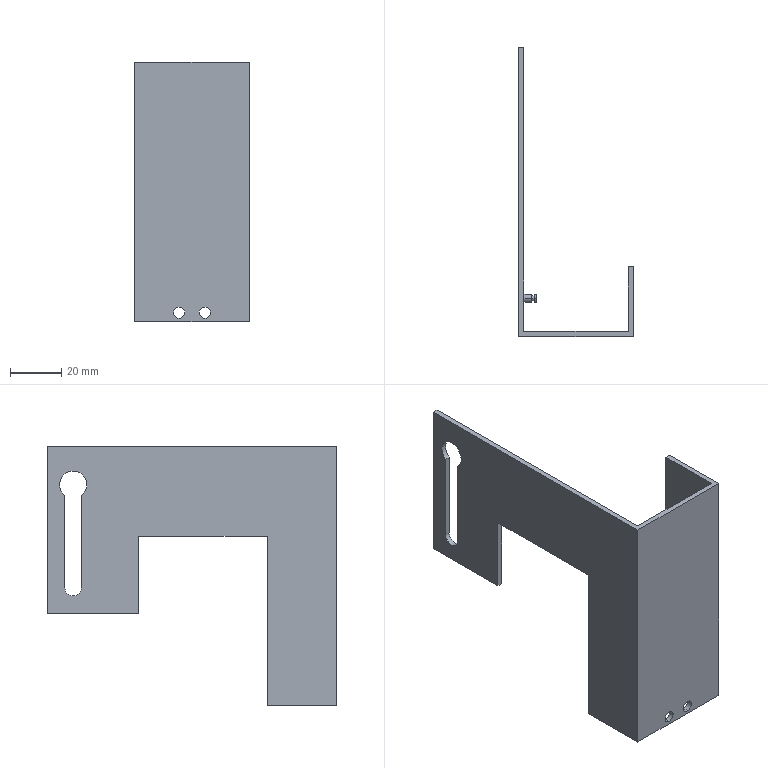Part | SolidWorks | features BaseBody 1 | 1 solid | 32 faces | box 44.5 x 112.5 x 101 mm | volume 26509 mm3 | plane 19 | cylinder 13 | commonest cylinder face diameters 3 x4 4.4 x4 2 x2 10.6 x2 6.5 x1
STEP:
#1=CARTESIAN_POINT('',(901.696,-4295.973,965.271));
#2=VERTEX_POINT('',#1);
#3=CARTESIAN_POINT('',(901.696,-4292.723,955.785));
#4=VERTEX_POINT('',#3);
#5=CARTESIAN_POINT('',(901.696,-4295.973,959.971));
#6=DIRECTION('',(-1.,0.,0.));
#7=DIRECTION('',(0.,0.,1.));
#8=AXIS2_PLACEMENT_3D('',#5,#6,#7);
#9=CIRCLE('',#8,5.3);
#10=EDGE_CURVE('',#2,#4,#9,.T.);
#11=ORIENTED_EDGE('',*,*,#10,.F.);
#12=CARTESIAN_POINT('',(899.696,-4295.973,965.271));
#13=VERTEX_POINT('',#12);
#14=CARTESIAN_POINT('',(922.28,-4295.973,965.271));
#15=DIRECTION('',(-1.,0.,0.));
#16=VECTOR('',#15,1000.);
#17=LINE('',#14,#16);
#18=EDGE_CURVE('',#2,#13,#17,.T.);
#19=ORIENTED_EDGE('',*,*,#18,.T.);
#20=CARTESIAN_POINT('',(899.696,-4292.723,955.785));
#21=VERTEX_POINT('',#20);
#22=CARTESIAN_POINT('',(899.696,-4295.973,959.971));
#23=DIRECTION('',(1.,0.,0.));
#24=DIRECTION('',(0.,0.,1.));
#25=AXIS2_PLACEMENT_3D('',#22,#23,#24);
#26=CIRCLE('',#25,5.3);
#27=EDGE_CURVE('',#21,#13,#26,.T.);
#28=ORIENTED_EDGE('',*,*,#27,.F.);
#29=CARTESIAN_POINT('',(973.716,-4292.723,955.785));
#30=DIRECTION('',(1.,0.,0.));
#31=VECTOR('',#30,1000.);
#32=LINE('',#29,#31);
#33=EDGE_CURVE('',#21,#4,#32,.T.);
#34=ORIENTED_EDGE('',*,*,#33,.T.);
#35=EDGE_LOOP('',(#11,#19,#28,#34));
#36=FACE_OUTER_BOUND('',#35,.T.);
#37=CARTESIAN_POINT('',(922.28,-4295.973,959.971));
#38=DIRECTION('',(-1.,0.,0.));
#39=DIRECTION('',(0.,0.,1.));
#40=AXIS2_PLACEMENT_3D('',#37,#38,#39);
#41=CYLINDRICAL_SURFACE('',#40,5.3);
#42=ADVANCED_FACE('',(#36),#41,.F.);
#43=CARTESIAN_POINT('',(916.941,-4396.473,879.671));
#44=VERTEX_POINT('',#43);
#45=CARTESIAN_POINT('',(916.941,-4396.473,875.271));
#46=VERTEX_POINT('',#45);
#47=CARTESIAN_POINT('',(916.941,-4396.473,877.471));
#48=DIRECTION('',(0.,-1.,0.));
#49=DIRECTION('',(0.,0.,-1.));
#50=AXIS2_PLACEMENT_3D('',#47,#48,#49);
#51=CIRCLE('',#50,2.2);
#52=EDGE_CURVE('',#44,#46,#51,.T.);
#53=ORIENTED_EDGE('',*,*,#52,.F.);
#54=CARTESIAN_POINT('',(916.941,-4398.473,879.671));
#55=VERTEX_POINT('',#54);
#56=CARTESIAN_POINT('',(916.941,-4401.568,879.671));
#57=DIRECTION('',(0.,-1.,0.));
#58=VECTOR('',#57,1000.);
#59=LINE('',#56,#58);
#60=EDGE_CURVE('',#44,#55,#59,.T.);
#61=ORIENTED_EDGE('',*,*,#60,.T.);
#62=CARTESIAN_POINT('',(916.941,-4398.473,875.271));
#63=VERTEX_POINT('',#62);
#64=CARTESIAN_POINT('',(916.941,-4398.473,877.471));
#65=DIRECTION('',(0.,1.,0.));
#66=DIRECTION('',(0.,0.,-1.));
#67=AXIS2_PLACEMENT_3D('',#64,#65,#66);
#68=CIRCLE('',#67,2.2);
#69=EDGE_CURVE('',#63,#55,#68,.T.);
#70=ORIENTED_EDGE('',*,*,#69,.F.);
#71=CARTESIAN_POINT('',(916.941,-4401.568,875.271));
#72=DIRECTION('',(0.,-1.,0.));
#73=VECTOR('',#72,1000.);
#74=LINE('',#71,#73);
#75=EDGE_CURVE('',#46,#63,#74,.T.);
#76=ORIENTED_EDGE('',*,*,#75,.F.);
#77=EDGE_LOOP('',(#53,#61,#70,#76));
#78=FACE_OUTER_BOUND('',#77,.T.);
#79=CARTESIAN_POINT('',(916.941,-4401.568,877.471));
#80=DIRECTION('',(0.,-1.,0.));
#81=DIRECTION('',(0.,0.,-1.));
#82=AXIS2_PLACEMENT_3D('',#79,#80,#81);
#83=CYLINDRICAL_SURFACE('',#82,2.2);
#84=ADVANCED_FACE('',(#78),#83,.F.);
#85=CARTESIAN_POINT('',(926.941,-4396.473,879.671));
#86=VERTEX_POINT('',#85);
#87=CARTESIAN_POINT('',(926.941,-4396.473,875.271));
#88=VERTEX_POINT('',#87);
#89=CARTESIAN_POINT('',(926.941,-4396.473,877.471));
#90=DIRECTION('',(0.,-1.,0.));
#91=DIRECTION('',(0.,0.,-1.));
#92=AXIS2_PLACEMENT_3D('',#89,#90,#91);
#93=CIRCLE('',#92,2.2);
#94=EDGE_CURVE('',#86,#88,#93,.T.);
#95=ORIENTED_EDGE('',*,*,#94,.F.);
#96=CARTESIAN_POINT('',(926.941,-4398.473,879.671));
#97=VERTEX_POINT('',#96);
#98=CARTESIAN_POINT('',(926.941,-4401.568,879.671));
#99=DIRECTION('',(0.,-1.,0.));
#100=VECTOR('',#99,1000.);
#101=LINE('',#98,#100);
#102=EDGE_CURVE('',#86,#97,#101,.T.);
#103=ORIENTED_EDGE('',*,*,#102,.T.);
#104=CARTESIAN_POINT('',(926.941,-4398.473,875.271));
#105=VERTEX_POINT('',#104);
#106=CARTESIAN_POINT('',(926.941,-4398.473,877.471));
#107=DIRECTION('',(0.,1.,0.));
#108=DIRECTION('',(0.,0.,-1.));
#109=AXIS2_PLACEMENT_3D('',#106,#107,#108);
#110=CIRCLE('',#109,2.2);
#111=EDGE_CURVE('',#105,#97,#110,.T.);
#112=ORIENTED_EDGE('',*,*,#111,.F.);
#113=CARTESIAN_POINT('',(926.941,-4401.568,875.271));
#114=DIRECTION('',(0.,-1.,0.));
#115=VECTOR('',#114,1000.);
#116=LINE('',#113,#115);
#117=EDGE_CURVE('',#88,#105,#116,.T.);
#118=ORIENTED_EDGE('',*,*,#117,.F.);
#119=EDGE_LOOP('',(#95,#103,#112,#118));
#120=FACE_OUTER_BOUND('',#119,.T.);
#121=CARTESIAN_POINT('',(926.941,-4401.568,877.471));
#122=DIRECTION('',(0.,-1.,0.));
#123=DIRECTION('',(0.,0.,-1.));
#124=AXIS2_PLACEMENT_3D('',#121,#122,#123);
#125=CYLINDRICAL_SURFACE('',#124,2.2);
#126=ADVANCED_FACE('',(#120),#125,.F.);
#127=CARTESIAN_POINT('',(904.696,-4383.47,878.971));
#128=VERTEX_POINT('',#127);
#129=CARTESIAN_POINT('',(904.696,-4383.47,875.971));
#130=VERTEX_POINT('',#129);
#131=CARTESIAN_POINT('',(904.696,-4383.47,877.471));
#132=DIRECTION('',(-1.,0.,0.));
#133=DIRECTION('',(0.,0.,1.));
#134=AXIS2_PLACEMENT_3D('',#131,#132,#133);
#135=CIRCLE('',#134,1.5);
#136=EDGE_CURVE('',#128,#130,#135,.T.);
#137=ORIENTED_EDGE('',*,*,#136,.T.);
#138=CARTESIAN_POINT('',(901.696,-4383.47,875.971));
#139=VERTEX_POINT('',#138);
#140=CARTESIAN_POINT('',(903.696,-4383.47,875.971));
#141=DIRECTION('',(-1.,0.,0.));
#142=VECTOR('',#141,1000.);
#143=LINE('',#140,#142);
#144=EDGE_CURVE('',#130,#139,#143,.T.);
#145=ORIENTED_EDGE('',*,*,#144,.T.);
#146=CARTESIAN_POINT('',(901.696,-4383.47,878.971));
#147=VERTEX_POINT('',#146);
#148=CARTESIAN_POINT('',(901.696,-4383.47,877.471));
#149=DIRECTION('',(-1.,0.,0.));
#150=DIRECTION('',(0.,0.,1.));
#151=AXIS2_PLACEMENT_3D('',#148,#149,#150);
#152=CIRCLE('',#151,1.5);
#153=EDGE_CURVE('',#147,#139,#152,.T.);
#154=ORIENTED_EDGE('',*,*,#153,.F.);
#155=CARTESIAN_POINT('',(903.696,-4383.47,878.971));
#156=DIRECTION('',(-1.,0.,0.));
#157=VECTOR('',#156,1000.);
#158=LINE('',#155,#157);
#159=EDGE_CURVE('',#128,#147,#158,.T.);
#160=ORIENTED_EDGE('',*,*,#159,.F.);
#161=EDGE_LOOP('',(#137,#145,#154,#160));
#162=FACE_OUTER_BOUND('',#161,.T.);
#163=CARTESIAN_POINT('',(903.696,-4383.47,877.471));
#164=DIRECTION('',(-1.,0.,0.));
#165=DIRECTION('',(0.,0.,1.));
#166=AXIS2_PLACEMENT_3D('',#163,#164,#165);
#167=CYLINDRICAL_SURFACE('',#166,1.5);
#168=ADVANCED_FACE('',(#162),#167,.T.);
#169=CARTESIAN_POINT('',(905.696,-4383.47,876.471));
#170=VERTEX_POINT('',#169);
#171=CARTESIAN_POINT('',(905.696,-4383.47,878.471));
#172=VERTEX_POINT('',#171);
#173=CARTESIAN_POINT('',(905.696,-4383.47,877.471));
#174=DIRECTION('',(1.,0.,0.));
#175=DIRECTION('',(0.,0.,1.));
#176=AXIS2_PLACEMENT_3D('',#173,#174,#175);
#177=CIRCLE('',#176,1.);
#178=EDGE_CURVE('',#170,#172,#177,.T.);
#179=ORIENTED_EDGE('',*,*,#178,.F.);
#180=CARTESIAN_POINT('',(904.696,-4383.47,876.471));
#181=VERTEX_POINT('',#180);
#182=CARTESIAN_POINT('',(905.696,-4383.47,876.471));
#183=DIRECTION('',(-1.,0.,0.));
#184=VECTOR('',#183,1000.);
#185=LINE('',#182,#184);
#186=EDGE_CURVE('',#170,#181,#185,.T.);
#187=ORIENTED_EDGE('',*,*,#186,.T.);
#188=CARTESIAN_POINT('',(904.696,-4383.47,878.471));
#189=VERTEX_POINT('',#188);
#190=CARTESIAN_POINT('',(904.696,-4383.47,877.471));
#191=DIRECTION('',(1.,0.,0.));
#192=DIRECTION('',(0.,0.,1.));
#193=AXIS2_PLACEMENT_3D('',#190,#191,#192);
#194=CIRCLE('',#193,1.);
#195=EDGE_CURVE('',#181,#189,#194,.T.);
#196=ORIENTED_EDGE('',*,*,#195,.T.);
#197=CARTESIAN_POINT('',(905.696,-4383.47,878.471));
#198=DIRECTION('',(-1.,0.,0.));
#199=VECTOR('',#198,1000.);
#200=LINE('',#197,#199);
#201=EDGE_CURVE('',#172,#189,#200,.T.);
#202=ORIENTED_EDGE('',*,*,#201,.F.);
#203=EDGE_LOOP('',(#179,#187,#196,#202));
#204=FACE_OUTER_BOUND('',#203,.T.);
#205=CARTESIAN_POINT('',(905.696,-4383.47,877.471));
#206=DIRECTION('',(-1.,0.,0.));
#207=DIRECTION('',(0.,0.,1.));
#208=AXIS2_PLACEMENT_3D('',#205,#206,#207);
#209=CYLINDRICAL_SURFACE('',#208,1.);
#210=ADVANCED_FACE('',(#204),#209,.T.);
#211=CARTESIAN_POINT('',(906.696,-4383.47,878.971));
#212=VERTEX_POINT('',#211);
#213=CARTESIAN_POINT('',(906.696,-4383.47,875.971));
#214=VERTEX_POINT('',#213);
#215=CARTESIAN_POINT('',(906.696,-4383.47,877.471));
#216=DIRECTION('',(-1.,0.,0.));
#217=DIRECTION('',(0.,0.,1.));
#218=AXIS2_PLACEMENT_3D('',#215,#216,#217);
#219=CIRCLE('',#218,1.5);
#220=EDGE_CURVE('',#212,#214,#219,.T.);
#221=ORIENTED_EDGE('',*,*,#220,.T.);
#222=CARTESIAN_POINT('',(905.696,-4383.47,875.971));
#223=VERTEX_POINT('',#222);
#224=CARTESIAN_POINT('',(903.696,-4383.47,875.971));
#225=DIRECTION('',(-1.,0.,0.));
#226=VECTOR('',#225,1000.);
#227=LINE('',#224,#226);
#228=EDGE_CURVE('',#214,#223,#227,.T.);
#229=ORIENTED_EDGE('',*,*,#228,.T.);
#230=CARTESIAN_POINT('',(905.696,-4383.47,878.971));
#231=VERTEX_POINT('',#230);
#232=CARTESIAN_POINT('',(905.696,-4383.47,877.471));
#233=DIRECTION('',(-1.,0.,0.));
#234=DIRECTION('',(0.,0.,1.));
#235=AXIS2_PLACEMENT_3D('',#232,#233,#234);
#236=CIRCLE('',#235,1.5);
#237=EDGE_CURVE('',#231,#223,#236,.T.);
#238=ORIENTED_EDGE('',*,*,#237,.F.);
#239=CARTESIAN_POINT('',(903.696,-4383.47,878.971));
#240=DIRECTION('',(-1.,0.,0.));
#241=VECTOR('',#240,1000.);
#242=LINE('',#239,#241);
#243=EDGE_CURVE('',#212,#231,#242,.T.);
#244=ORIENTED_EDGE('',*,*,#243,.F.);
#245=EDGE_LOOP('',(#221,#229,#238,#244));
#246=FACE_OUTER_BOUND('',#245,.T.);
#247=CARTESIAN_POINT('',(903.696,-4383.47,877.471));
#248=DIRECTION('',(-1.,0.,0.));
#249=DIRECTION('',(0.,0.,1.));
#250=AXIS2_PLACEMENT_3D('',#247,#248,#249);
#251=CYLINDRICAL_SURFACE('',#250,1.5);
#252=ADVANCED_FACE('',(#246),#251,.T.);
#253=CARTESIAN_POINT('',(899.696,-4285.973,974.971));
#254=VERTEX_POINT('',#253);
#255=CARTESIAN_POINT('',(899.696,-4285.973,909.971));
#256=VERTEX_POINT('',#255);
#257=CARTESIAN_POINT('',(899.696,-4285.973,874.971));
#258=DIRECTION('',(0.,0.,-1.));
#259=VECTOR('',#258,1000.);
#260=LINE('',#257,#259);
#261=EDGE_CURVE('',#254,#256,#260,.T.);
#262=ORIENTED_EDGE('',*,*,#261,.T.);
#263=CARTESIAN_POINT('',(899.696,-4321.473,909.971));
#264=VERTEX_POINT('',#263);
#265=CARTESIAN_POINT('',(899.696,-4398.473,909.971));
#266=DIRECTION('',(0.,-1.,0.));
#267=VECTOR('',#266,1000.);
#268=LINE('',#265,#267);
#269=EDGE_CURVE('',#256,#264,#268,.T.);
#270=ORIENTED_EDGE('',*,*,#269,.T.);
#271=CARTESIAN_POINT('',(899.696,-4321.473,939.971));
#272=VERTEX_POINT('',#271);
#273=CARTESIAN_POINT('',(899.696,-4321.473,874.971));
#274=DIRECTION('',(0.,0.,1.));
#275=VECTOR('',#274,1000.);
#276=LINE('',#273,#275);
#277=EDGE_CURVE('',#264,#272,#276,.T.);
#278=ORIENTED_EDGE('',*,*,#277,.T.);
#279=CARTESIAN_POINT('',(899.696,-4371.473,939.971));
#280=VERTEX_POINT('',#279);
#281=CARTESIAN_POINT('',(899.696,-4398.473,939.971));
#282=DIRECTION('',(0.,-1.,0.));
#283=VECTOR('',#282,1000.);
#284=LINE('',#281,#283);
#285=EDGE_CURVE('',#272,#280,#284,.T.);
#286=ORIENTED_EDGE('',*,*,#285,.T.);
#287=CARTESIAN_POINT('',(899.696,-4371.473,873.971));
#288=VERTEX_POINT('',#287);
#289=CARTESIAN_POINT('',(899.696,-4371.473,874.971));
#290=DIRECTION('',(0.,0.,-1.));
#291=VECTOR('',#290,1000.);
#292=LINE('',#289,#291);
#293=EDGE_CURVE('',#280,#288,#292,.T.);
#294=ORIENTED_EDGE('',*,*,#293,.T.);
#295=CARTESIAN_POINT('',(899.696,-4398.473,873.971));
#296=VERTEX_POINT('',#295);
#297=CARTESIAN_POINT('',(899.696,-4398.473,873.971));
#298=DIRECTION('',(0.,-1.,0.));
#299=VECTOR('',#298,1000.);
#300=LINE('',#297,#299);
#301=EDGE_CURVE('',#288,#296,#300,.T.);
#302=ORIENTED_EDGE('',*,*,#301,.T.);
#303=CARTESIAN_POINT('',(899.696,-4398.473,974.971));
#304=VERTEX_POINT('',#303);
#305=CARTESIAN_POINT('',(899.696,-4398.473,874.971));
#306=DIRECTION('',(0.,0.,1.));
#307=VECTOR('',#306,1000.);
#308=LINE('',#305,#307);
#309=EDGE_CURVE('',#296,#304,#308,.T.);
#310=ORIENTED_EDGE('',*,*,#309,.T.);
#311=CARTESIAN_POINT('',(899.696,-4398.473,974.971));
#312=DIRECTION('',(0.,1.,0.));
#313=VECTOR('',#312,1000.);
#314=LINE('',#311,#313);
#315=EDGE_CURVE('',#304,#254,#314,.T.);
#316=ORIENTED_EDGE('',*,*,#315,.T.);
#317=EDGE_LOOP('',(#262,#270,#278,#286,#294,#302,#310,#316));
#318=FACE_OUTER_BOUND('',#317,.T.);
#319=CARTESIAN_POINT('',(899.696,-4299.223,919.971));
#320=VERTEX_POINT('',#319);
#321=CARTESIAN_POINT('',(899.696,-4292.723,919.971));
#322=VERTEX_POINT('',#321);
#323=CARTESIAN_POINT('',(899.696,-4295.973,919.971));
#324=DIRECTION('',(1.,0.,0.));
#325=DIRECTION('',(0.,0.,1.));
#326=AXIS2_PLACEMENT_3D('',#323,#324,#325);
#327=CIRCLE('',#326,3.25);
#328=EDGE_CURVE('',#320,#322,#327,.T.);
#329=ORIENTED_EDGE('',*,*,#328,.T.);
#330=CARTESIAN_POINT('',(899.696,-4292.723,874.971));
#331=DIRECTION('',(0.,0.,1.));
#332=VECTOR('',#331,1000.);
#333=LINE('',#330,#332);
#334=EDGE_CURVE('',#322,#21,#333,.T.);
#335=ORIENTED_EDGE('',*,*,#334,.T.);
#336=ORIENTED_EDGE('',*,*,#27,.T.);
#337=CARTESIAN_POINT('',(899.696,-4299.223,955.785));
#338=VERTEX_POINT('',#337);
#339=CARTESIAN_POINT('',(899.696,-4295.973,959.971));
#340=DIRECTION('',(1.,0.,0.));
#341=DIRECTION('',(0.,0.,1.));
#342=AXIS2_PLACEMENT_3D('',#339,#340,#341);
#343=CIRCLE('',#342,5.3);
#344=EDGE_CURVE('',#13,#338,#343,.T.);
#345=ORIENTED_EDGE('',*,*,#344,.T.);
#346=CARTESIAN_POINT('',(899.696,-4299.223,874.971));
#347=DIRECTION('',(0.,0.,-1.));
#348=VECTOR('',#347,1000.);
#349=LINE('',#346,#348);
#350=EDGE_CURVE('',#338,#320,#349,.T.);
#351=ORIENTED_EDGE('',*,*,#350,.T.);
#352=EDGE_LOOP('',(#329,#335,#336,#345,#351));
#353=FACE_BOUND('',#352,.T.);
#354=CARTESIAN_POINT('',(899.696,-4398.473,874.971));
#355=DIRECTION('',(-1.,0.,0.));
#356=DIRECTION('',(0.,0.,1.));
#357=AXIS2_PLACEMENT_3D('',#354,#355,#356);
#358=PLANE('',#357);
#359=ADVANCED_FACE('',(#318,#353),#358,.T.);
#360=ORIENTED_EDGE('',*,*,#269,.F.);
#361=CARTESIAN_POINT('',(901.696,-4285.973,909.971));
#362=VERTEX_POINT('',#361);
#363=CARTESIAN_POINT('',(1601.029,-4285.973,909.971));
#364=DIRECTION('',(-1.,0.,0.));
#365=VECTOR('',#364,1000.);
#366=LINE('',#363,#365);
#367=EDGE_CURVE('',#362,#256,#366,.T.);
#368=ORIENTED_EDGE('',*,*,#367,.F.);
#369=CARTESIAN_POINT('',(901.696,-4321.473,909.971));
#370=VERTEX_POINT('',#369);
#371=CARTESIAN_POINT('',(901.696,-4271.473,909.971));
#372=DIRECTION('',(0.,1.,0.));
#373=VECTOR('',#372,1000.);
#374=LINE('',#371,#373);
#375=EDGE_CURVE('',#370,#362,#374,.T.);
#376=ORIENTED_EDGE('',*,*,#375,.F.);
#377=CARTESIAN_POINT('',(1601.029,-4321.473,909.971));
#378=DIRECTION('',(1.,0.,0.));
#379=VECTOR('',#378,1000.);
#380=LINE('',#377,#379);
#381=EDGE_CURVE('',#264,#370,#380,.T.);
#382=ORIENTED_EDGE('',*,*,#381,.F.);
#383=EDGE_LOOP('',(#360,#368,#376,#382));
#384=FACE_OUTER_BOUND('',#383,.T.);
#385=CARTESIAN_POINT('',(1601.029,-4271.473,909.971));
#386=DIRECTION('',(0.,0.,1.));
#387=DIRECTION('',(1.,0.,0.));
#388=AXIS2_PLACEMENT_3D('',#385,#386,#387);
#389=PLANE('',#388);
#390=ADVANCED_FACE('',(#384),#389,.F.);
#391=CARTESIAN_POINT('',(901.696,-4285.973,974.971));
#392=VERTEX_POINT('',#391);
#393=CARTESIAN_POINT('',(899.696,-4285.973,974.971));
#394=DIRECTION('',(1.,0.,0.));
#395=VECTOR('',#394,1000.);
#396=LINE('',#393,#395);
#397=EDGE_CURVE('',#254,#392,#396,.T.);
#398=ORIENTED_EDGE('',*,*,#397,.T.);
#399=CARTESIAN_POINT('',(901.696,-4285.973,874.971));
#400=DIRECTION('',(0.,0.,-1.));
#401=VECTOR('',#400,1000.);
#402=LINE('',#399,#401);
#403=EDGE_CURVE('',#392,#362,#402,.T.);
#404=ORIENTED_EDGE('',*,*,#403,.T.);
#405=ORIENTED_EDGE('',*,*,#367,.T.);
#406=ORIENTED_EDGE('',*,*,#261,.F.);
#407=EDGE_LOOP('',(#398,#404,#405,#406));
#408=FACE_OUTER_BOUND('',#407,.T.);
#409=CARTESIAN_POINT('',(899.696,-4285.973,874.971));
#410=DIRECTION('',(0.,1.,0.));
#411=DIRECTION('',(0.,0.,1.));
#412=AXIS2_PLACEMENT_3D('',#409,#410,#411);
#413=PLANE('',#412);
#414=ADVANCED_FACE('',(#408),#413,.T.);
#415=CARTESIAN_POINT('',(942.196,-4371.473,974.971));
#416=VERTEX_POINT('',#415);
#417=CARTESIAN_POINT('',(942.196,-4396.473,974.971));
#418=VERTEX_POINT('',#417);
#419=CARTESIAN_POINT('',(942.196,-4360.722,974.971));
#420=DIRECTION('',(0.,-1.,0.));
#421=VECTOR('',#420,1000.);
#422=LINE('',#419,#421);
#423=EDGE_CURVE('',#416,#418,#422,.T.);
#424=ORIENTED_EDGE('',*,*,#423,.T.);
#425=CARTESIAN_POINT('',(901.696,-4396.473,974.971));
#426=VERTEX_POINT('',#425);
#427=CARTESIAN_POINT('',(911.963,-4396.473,974.971));
#428=DIRECTION('',(-1.,0.,0.));
#429=VECTOR('',#428,1000.);
#430=LINE('',#427,#429);
#431=EDGE_CURVE('',#418,#426,#430,.T.);
#432=ORIENTED_EDGE('',*,*,#431,.T.);
#433=CARTESIAN_POINT('',(901.696,-4360.722,974.971));
#434=DIRECTION('',(0.,1.,0.));
#435=VECTOR('',#434,1000.);
#436=LINE('',#433,#435);
#437=EDGE_CURVE('',#426,#392,#436,.T.);
#438=ORIENTED_EDGE('',*,*,#437,.T.);
#439=ORIENTED_EDGE('',*,*,#397,.F.);
#440=ORIENTED_EDGE('',*,*,#315,.F.);
#441=CARTESIAN_POINT('',(944.196,-4398.473,974.971));
#442=VERTEX_POINT('',#441);
#443=CARTESIAN_POINT('',(911.963,-4398.473,974.971));
#444=DIRECTION('',(1.,0.,0.));
#445=VECTOR('',#444,1000.);
#446=LINE('',#443,#445);
#447=EDGE_CURVE('',#304,#442,#446,.T.);
#448=ORIENTED_EDGE('',*,*,#447,.T.);
#449=CARTESIAN_POINT('',(944.196,-4371.473,974.971));
#450=VERTEX_POINT('',#449);
#451=CARTESIAN_POINT('',(944.196,-4360.722,974.971));
#452=DIRECTION('',(0.,1.,0.));
#453=VECTOR('',#452,1000.);
#454=LINE('',#451,#453);
#455=EDGE_CURVE('',#442,#450,#454,.T.);
#456=ORIENTED_EDGE('',*,*,#455,.T.);
#457=CARTESIAN_POINT('',(911.963,-4371.473,974.971));
#458=DIRECTION('',(-1.,0.,0.));
#459=VECTOR('',#458,1000.);
#460=LINE('',#457,#459);
#461=EDGE_CURVE('',#450,#416,#460,.T.);
#462=ORIENTED_EDGE('',*,*,#461,.T.);
#463=EDGE_LOOP('',(#424,#432,#438,#439,#440,#448,#456,#462));
#464=FACE_OUTER_BOUND('',#463,.T.);
#465=CARTESIAN_POINT('',(911.963,-4360.722,974.971));
#466=DIRECTION('',(0.,0.,1.));
#467=DIRECTION('',(1.,0.,0.));
#468=AXIS2_PLACEMENT_3D('',#465,#466,#467);
#469=PLANE('',#468);
#470=ADVANCED_FACE('',(#464),#469,.T.);
#471=CARTESIAN_POINT('',(944.196,-4398.473,873.971));
#472=VERTEX_POINT('',#471);
#473=CARTESIAN_POINT('',(944.196,-4398.473,873.971));
#474=DIRECTION('',(1.,0.,0.));
#475=VECTOR('',#474,1000.);
#476=LINE('',#473,#475);
#477=EDGE_CURVE('',#296,#472,#476,.T.);
#478=ORIENTED_EDGE('',*,*,#477,.T.);
#479=CARTESIAN_POINT('',(944.196,-4398.473,873.971));
#480=DIRECTION('',(0.,0.,1.));
#481=VECTOR('',#480,1000.);
#482=LINE('',#479,#481);
#483=EDGE_CURVE('',#472,#442,#482,.T.);
#484=ORIENTED_EDGE('',*,*,#483,.T.);
#485=ORIENTED_EDGE('',*,*,#447,.F.);
#486=ORIENTED_EDGE('',*,*,#309,.F.);
#487=EDGE_LOOP('',(#478,#484,#485,#486));
#488=FACE_OUTER_BOUND('',#487,.T.);
#489=ORIENTED_EDGE('',*,*,#69,.T.);
#490=CARTESIAN_POINT('',(916.941,-4398.473,877.471));
#491=DIRECTION('',(0.,1.,0.));
#492=DIRECTION('',(0.,0.,-1.));
#493=AXIS2_PLACEMENT_3D('',#490,#491,#492);
#494=CIRCLE('',#493,2.2);
#495=EDGE_CURVE('',#55,#63,#494,.T.);
#496=ORIENTED_EDGE('',*,*,#495,.T.);
#497=EDGE_LOOP('',(#489,#496));
#498=FACE_BOUND('',#497,.T.);
#499=ORIENTED_EDGE('',*,*,#111,.T.);
#500=CARTESIAN_POINT('',(926.941,-4398.473,877.471));
#501=DIRECTION('',(0.,1.,0.));
#502=DIRECTION('',(0.,0.,-1.));
#503=AXIS2_PLACEMENT_3D('',#500,#501,#502);
#504=CIRCLE('',#503,2.2);
#505=EDGE_CURVE('',#97,#105,#504,.T.);
#506=ORIENTED_EDGE('',*,*,#505,.T.);
#507=EDGE_LOOP('',(#499,#506));
#508=FACE_BOUND('',#507,.T.);
#509=CARTESIAN_POINT('',(944.196,-4398.473,873.971));
#510=DIRECTION('',(0.,-1.,0.));
#511=DIRECTION('',(0.,0.,-1.));
#512=AXIS2_PLACEMENT_3D('',#509,#510,#511);
#513=PLANE('',#512);
#514=ADVANCED_FACE('',(#488,#498,#508),#513,.T.);
#515=CARTESIAN_POINT('',(942.196,-4371.473,873.971));
#516=VERTEX_POINT('',#515);
#517=CARTESIAN_POINT('',(942.196,-4396.473,873.971));
#518=VERTEX_POINT('',#517);
#519=CARTESIAN_POINT('',(942.196,-4360.722,873.971));
#520=DIRECTION('',(0.,-1.,0.));
#521=VECTOR('',#520,1000.);
#522=LINE('',#519,#521);
#523=EDGE_CURVE('',#516,#518,#522,.T.);
#524=ORIENTED_EDGE('',*,*,#523,.F.);
#525=CARTESIAN_POINT('',(944.196,-4371.473,873.971));
#526=VERTEX_POINT('',#525);
#527=CARTESIAN_POINT('',(911.963,-4371.473,873.971));
#528=DIRECTION('',(-1.,0.,0.));
#529=VECTOR('',#528,1000.);
#530=LINE('',#527,#529);
#531=EDGE_CURVE('',#526,#516,#530,.T.);
#532=ORIENTED_EDGE('',*,*,#531,.F.);
#533=CARTESIAN_POINT('',(944.196,-4360.722,873.971));
#534=DIRECTION('',(0.,1.,0.));
#535=VECTOR('',#534,1000.);
#536=LINE('',#533,#535);
#537=EDGE_CURVE('',#472,#526,#536,.T.);
#538=ORIENTED_EDGE('',*,*,#537,.F.);
#539=ORIENTED_EDGE('',*,*,#477,.F.);
#540=ORIENTED_EDGE('',*,*,#301,.F.);
#541=CARTESIAN_POINT('',(901.696,-4371.473,873.971));
#542=VERTEX_POINT('',#541);
#543=CARTESIAN_POINT('',(911.963,-4371.473,873.971));
#544=DIRECTION('',(-1.,0.,0.));
#545=VECTOR('',#544,1000.);
#546=LINE('',#543,#545);
#547=EDGE_CURVE('',#542,#288,#546,.T.);
#548=ORIENTED_EDGE('',*,*,#547,.F.);
#549=CARTESIAN_POINT('',(901.696,-4396.473,873.971));
#550=VERTEX_POINT('',#549);
#551=CARTESIAN_POINT('',(901.696,-4360.722,873.971));
#552=DIRECTION('',(0.,1.,0.));
#553=VECTOR('',#552,1000.);
#554=LINE('',#551,#553);
#555=EDGE_CURVE('',#550,#542,#554,.T.);
#556=ORIENTED_EDGE('',*,*,#555,.F.);
#557=CARTESIAN_POINT('',(911.963,-4396.473,873.971));
#558=DIRECTION('',(-1.,0.,0.));
#559=VECTOR('',#558,1000.);
#560=LINE('',#557,#559);
#561=EDGE_CURVE('',#518,#550,#560,.T.);
#562=ORIENTED_EDGE('',*,*,#561,.F.);
#563=EDGE_LOOP('',(#524,#532,#538,#539,#540,#548,#556,#562));
#564=FACE_OUTER_BOUND('',#563,.T.);
#565=CARTESIAN_POINT('',(911.963,-4360.722,873.971));
#566=DIRECTION('',(0.,0.,1.));
#567=DIRECTION('',(1.,0.,0.));
#568=AXIS2_PLACEMENT_3D('',#565,#566,#567);
#569=PLANE('',#568);
#570=ADVANCED_FACE('',(#564),#569,.F.);
#571=ORIENTED_EDGE('',*,*,#547,.T.);
#572=ORIENTED_EDGE('',*,*,#293,.F.);
#573=CARTESIAN_POINT('',(901.696,-4371.473,939.971));
#574=VERTEX_POINT('',#573);
#575=CARTESIAN_POINT('',(1601.029,-4371.473,939.971));
#576=DIRECTION('',(-1.,0.,0.));
#577=VECTOR('',#576,1000.);
#578=LINE('',#575,#577);
#579=EDGE_CURVE('',#574,#280,#578,.T.);
#580=ORIENTED_EDGE('',*,*,#579,.F.);
#581=CARTESIAN_POINT('',(901.696,-4371.473,909.971));
#582=DIRECTION('',(0.,0.,1.));
#583=VECTOR('',#582,1000.);
#584=LINE('',#581,#583);
#585=EDGE_CURVE('',#542,#574,#584,.T.);
#586=ORIENTED_EDGE('',*,*,#585,.F.);
#587=EDGE_LOOP('',(#571,#572,#580,#586));
#588=FACE_OUTER_BOUND('',#587,.T.);
#589=CARTESIAN_POINT('',(1601.029,-4371.473,909.971));
#590=DIRECTION('',(0.,-1.,0.));
#591=DIRECTION('',(0.,0.,-1.));
#592=AXIS2_PLACEMENT_3D('',#589,#590,#591);
#593=PLANE('',#592);
#594=ADVANCED_FACE('',(#588),#593,.F.);
#595=ORIENTED_EDGE('',*,*,#579,.T.);
#596=ORIENTED_EDGE('',*,*,#285,.F.);
#597=CARTESIAN_POINT('',(901.696,-4321.473,939.971));
#598=VERTEX_POINT('',#597);
#599=CARTESIAN_POINT('',(1019.248,-4321.473,939.971));
#600=DIRECTION('',(-1.,0.,0.));
#601=VECTOR('',#600,1000.);
#602=LINE('',#599,#601);
#603=EDGE_CURVE('',#598,#272,#602,.T.);
#604=ORIENTED_EDGE('',*,*,#603,.F.);
#605=CARTESIAN_POINT('',(901.696,-4351.473,939.971));
#606=DIRECTION('',(0.,1.,0.));
#607=VECTOR('',#606,1000.);
#608=LINE('',#605,#607);
#609=EDGE_CURVE('',#574,#598,#608,.T.);
#610=ORIENTED_EDGE('',*,*,#609,.F.);
#611=EDGE_LOOP('',(#595,#596,#604,#610));
#612=FACE_OUTER_BOUND('',#611,.T.);
#613=CARTESIAN_POINT('',(1019.248,-4351.473,939.971));
#614=DIRECTION('',(0.,0.,1.));
#615=DIRECTION('',(1.,0.,0.));
#616=AXIS2_PLACEMENT_3D('',#613,#614,#615);
#617=PLANE('',#616);
#618=ADVANCED_FACE('',(#612),#617,.F.);
#619=ORIENTED_EDGE('',*,*,#603,.T.);
#620=ORIENTED_EDGE('',*,*,#277,.F.);
#621=ORIENTED_EDGE('',*,*,#381,.T.);
#622=CARTESIAN_POINT('',(901.696,-4321.473,889.971));
#623=DIRECTION('',(0.,0.,-1.));
#624=VECTOR('',#623,1000.);
#625=LINE('',#622,#624);
#626=EDGE_CURVE('',#598,#370,#625,.T.);
#627=ORIENTED_EDGE('',*,*,#626,.F.);
#628=EDGE_LOOP('',(#619,#620,#621,#627));
#629=FACE_OUTER_BOUND('',#628,.T.);
#630=CARTESIAN_POINT('',(1019.248,-4321.473,889.971));
#631=DIRECTION('',(0.,1.,0.));
#632=DIRECTION('',(0.,0.,1.));
#633=AXIS2_PLACEMENT_3D('',#630,#631,#632);
#634=PLANE('',#633);
#635=ADVANCED_FACE('',(#629),#634,.F.);
#636=CARTESIAN_POINT('',(901.696,-4292.723,919.971));
#637=VERTEX_POINT('',#636);
#638=CARTESIAN_POINT('',(973.716,-4292.723,919.971));
#639=DIRECTION('',(-1.,0.,0.));
#640=VECTOR('',#639,1000.);
#641=LINE('',#638,#640);
#642=EDGE_CURVE('',#637,#322,#641,.T.);
#643=ORIENTED_EDGE('',*,*,#642,.F.);
#644=CARTESIAN_POINT('',(901.696,-4292.723,919.971));
#645=DIRECTION('',(0.,0.,-1.));
#646=VECTOR('',#645,1000.);
#647=LINE('',#644,#646);
#648=EDGE_CURVE('',#4,#637,#647,.T.);
#649=ORIENTED_EDGE('',*,*,#648,.F.);
#650=ORIENTED_EDGE('',*,*,#33,.F.);
#651=ORIENTED_EDGE('',*,*,#334,.F.);
#652=EDGE_LOOP('',(#643,#649,#650,#651));
#653=FACE_OUTER_BOUND('',#652,.T.);
#654=CARTESIAN_POINT('',(973.716,-4292.723,919.971));
#655=DIRECTION('',(0.,1.,0.));
#656=DIRECTION('',(0.,0.,1.));
#657=AXIS2_PLACEMENT_3D('',#654,#655,#656);
#658=PLANE('',#657);
#659=ADVANCED_FACE('',(#653),#658,.F.);
#660=CARTESIAN_POINT('',(901.696,-4299.223,919.971));
#661=VERTEX_POINT('',#660);
#662=CARTESIAN_POINT('',(973.716,-4299.223,919.971));
#663=DIRECTION('',(-1.,0.,0.));
#664=VECTOR('',#663,1000.);
#665=LINE('',#662,#664);
#666=EDGE_CURVE('',#661,#320,#665,.T.);
#667=ORIENTED_EDGE('',*,*,#666,.F.);
#668=CARTESIAN_POINT('',(901.696,-4295.973,919.971));
#669=DIRECTION('',(-1.,0.,0.));
#670=DIRECTION('',(0.,0.,1.));
#671=AXIS2_PLACEMENT_3D('',#668,#669,#670);
#672=CIRCLE('',#671,3.25);
#673=EDGE_CURVE('',#637,#661,#672,.T.);
#674=ORIENTED_EDGE('',*,*,#673,.F.);
#675=ORIENTED_EDGE('',*,*,#642,.T.);
#676=ORIENTED_EDGE('',*,*,#328,.F.);
#677=EDGE_LOOP('',(#667,#674,#675,#676));
#678=FACE_OUTER_BOUND('',#677,.T.);
#679=CARTESIAN_POINT('',(973.716,-4295.973,919.971));
#680=DIRECTION('',(-1.,0.,0.));
#681=DIRECTION('',(0.,0.,1.));
#682=AXIS2_PLACEMENT_3D('',#679,#680,#681);
#683=CYLINDRICAL_SURFACE('',#682,3.25);
#684=ADVANCED_FACE('',(#678),#683,.F.);
#685=CARTESIAN_POINT('',(901.696,-4299.223,955.785));
#686=VERTEX_POINT('',#685);
#687=CARTESIAN_POINT('',(973.716,-4299.223,955.785));
#688=DIRECTION('',(-1.,0.,0.));
#689=VECTOR('',#688,1000.);
#690=LINE('',#687,#689);
#691=EDGE_CURVE('',#686,#338,#690,.T.);
#692=ORIENTED_EDGE('',*,*,#691,.F.);
#693=CARTESIAN_POINT('',(901.696,-4299.223,959.971));
#694=DIRECTION('',(0.,0.,1.));
#695=VECTOR('',#694,1000.);
#696=LINE('',#693,#695);
#697=EDGE_CURVE('',#661,#686,#696,.T.);
#698=ORIENTED_EDGE('',*,*,#697,.F.);
#699=ORIENTED_EDGE('',*,*,#666,.T.);
#700=ORIENTED_EDGE('',*,*,#350,.F.);
#701=EDGE_LOOP('',(#692,#698,#699,#700));
#702=FACE_OUTER_BOUND('',#701,.T.);
#703=CARTESIAN_POINT('',(973.716,-4299.223,959.971));
#704=DIRECTION('',(0.,-1.,0.));
#705=DIRECTION('',(0.,0.,-1.));
#706=AXIS2_PLACEMENT_3D('',#703,#704,#705);
#707=PLANE('',#706);
#708=ADVANCED_FACE('',(#702),#707,.F.);
#709=ORIENTED_EDGE('',*,*,#18,.F.);
#710=CARTESIAN_POINT('',(901.696,-4295.973,959.971));
#711=DIRECTION('',(-1.,0.,0.));
#712=DIRECTION('',(0.,0.,1.));
#713=AXIS2_PLACEMENT_3D('',#710,#711,#712);
#714=CIRCLE('',#713,5.3);
#715=EDGE_CURVE('',#686,#2,#714,.T.);
#716=ORIENTED_EDGE('',*,*,#715,.F.);
#717=ORIENTED_EDGE('',*,*,#691,.T.);
#718=ORIENTED_EDGE('',*,*,#344,.F.);
#719=EDGE_LOOP('',(#709,#716,#717,#718));
#720=FACE_OUTER_BOUND('',#719,.T.);
#721=CARTESIAN_POINT('',(922.28,-4295.973,959.971));
#722=DIRECTION('',(-1.,0.,0.));
#723=DIRECTION('',(0.,0.,1.));
#724=AXIS2_PLACEMENT_3D('',#721,#722,#723);
#725=CYLINDRICAL_SURFACE('',#724,5.3);
#726=ADVANCED_FACE('',(#720),#725,.F.);
#727=ORIENTED_EDGE('',*,*,#153,.T.);
#728=CARTESIAN_POINT('',(901.696,-4383.47,877.471));
#729=DIRECTION('',(-1.,0.,0.));
#730=DIRECTION('',(0.,0.,1.));
#731=AXIS2_PLACEMENT_3D('',#728,#729,#730);
#732=CIRCLE('',#731,1.5);
#733=EDGE_CURVE('',#139,#147,#732,.T.);
#734=ORIENTED_EDGE('',*,*,#733,.T.);
#735=EDGE_LOOP('',(#727,#734));
#736=FACE_BOUND('',#735,.T.);
#737=ORIENTED_EDGE('',*,*,#585,.T.);
#738=ORIENTED_EDGE('',*,*,#609,.T.);
#739=ORIENTED_EDGE('',*,*,#626,.T.);
#740=ORIENTED_EDGE('',*,*,#375,.T.);
#741=ORIENTED_EDGE('',*,*,#403,.F.);
#742=ORIENTED_EDGE('',*,*,#437,.F.);
#743=CARTESIAN_POINT('',(901.696,-4396.473,874.971));
#744=DIRECTION('',(0.,0.,-1.));
#745=VECTOR('',#744,1000.);
#746=LINE('',#743,#745);
#747=EDGE_CURVE('',#426,#550,#746,.T.);
#748=ORIENTED_EDGE('',*,*,#747,.T.);
#749=ORIENTED_EDGE('',*,*,#555,.T.);
#750=EDGE_LOOP('',(#737,#738,#739,#740,#741,#742,#748,#749));
#751=FACE_OUTER_BOUND('',#750,.T.);
#752=ORIENTED_EDGE('',*,*,#673,.T.);
#753=ORIENTED_EDGE('',*,*,#697,.T.);
#754=ORIENTED_EDGE('',*,*,#715,.T.);
#755=ORIENTED_EDGE('',*,*,#10,.T.);
#756=ORIENTED_EDGE('',*,*,#648,.T.);
#757=EDGE_LOOP('',(#752,#753,#754,#755,#756));
#758=FACE_BOUND('',#757,.T.);
#759=CARTESIAN_POINT('',(901.696,-4285.973,874.971));
#760=DIRECTION('',(1.,0.,0.));
#761=DIRECTION('',(0.,0.,-1.));
#762=AXIS2_PLACEMENT_3D('',#759,#760,#761);
#763=PLANE('',#762);
#764=ADVANCED_FACE('',(#736,#751,#758),#763,.T.);
#765=ORIENTED_EDGE('',*,*,#431,.F.);
#766=CARTESIAN_POINT('',(942.196,-4396.473,872.971));
#767=DIRECTION('',(0.,0.,-1.));
#768=VECTOR('',#767,1000.);
#769=LINE('',#766,#768);
#770=EDGE_CURVE('',#418,#518,#769,.T.);
#771=ORIENTED_EDGE('',*,*,#770,.T.);
#772=ORIENTED_EDGE('',*,*,#561,.T.);
#773=ORIENTED_EDGE('',*,*,#747,.F.);
#774=EDGE_LOOP('',(#765,#771,#772,#773));
#775=FACE_OUTER_BOUND('',#774,.T.);
#776=CARTESIAN_POINT('',(916.941,-4396.473,877.471));
#777=DIRECTION('',(0.,-1.,0.));
#778=DIRECTION('',(0.,0.,-1.));
#779=AXIS2_PLACEMENT_3D('',#776,#777,#778);
#780=CIRCLE('',#779,2.2);
#781=EDGE_CURVE('',#46,#44,#780,.T.);
#782=ORIENTED_EDGE('',*,*,#781,.T.);
#783=ORIENTED_EDGE('',*,*,#52,.T.);
#784=EDGE_LOOP('',(#782,#783));
#785=FACE_BOUND('',#784,.T.);
#786=CARTESIAN_POINT('',(926.941,-4396.473,877.471));
#787=DIRECTION('',(0.,-1.,0.));
#788=DIRECTION('',(0.,0.,-1.));
#789=AXIS2_PLACEMENT_3D('',#786,#787,#788);
#790=CIRCLE('',#789,2.2);
#791=EDGE_CURVE('',#88,#86,#790,.T.);
#792=ORIENTED_EDGE('',*,*,#791,.T.);
#793=ORIENTED_EDGE('',*,*,#94,.T.);
#794=EDGE_LOOP('',(#792,#793));
#795=FACE_BOUND('',#794,.T.);
#796=CARTESIAN_POINT('',(911.946,-4396.473,872.971));
#797=DIRECTION('',(0.,1.,0.));
#798=DIRECTION('',(0.,0.,1.));
#799=AXIS2_PLACEMENT_3D('',#796,#797,#798);
#800=PLANE('',#799);
#801=ADVANCED_FACE('',(#775,#785,#795),#800,.T.);
#802=ORIENTED_EDGE('',*,*,#523,.T.);
#803=ORIENTED_EDGE('',*,*,#770,.F.);
#804=ORIENTED_EDGE('',*,*,#423,.F.);
#805=CARTESIAN_POINT('',(942.196,-4371.473,874.971));
#806=DIRECTION('',(0.,0.,-1.));
#807=VECTOR('',#806,1000.);
#808=LINE('',#805,#807);
#809=EDGE_CURVE('',#416,#516,#808,.T.);
#810=ORIENTED_EDGE('',*,*,#809,.T.);
#811=EDGE_LOOP('',(#802,#803,#804,#810));
#812=FACE_OUTER_BOUND('',#811,.T.);
#813=CARTESIAN_POINT('',(942.196,-4396.473,874.971));
#814=DIRECTION('',(-1.,0.,0.));
#815=DIRECTION('',(0.,0.,1.));
#816=AXIS2_PLACEMENT_3D('',#813,#814,#815);
#817=PLANE('',#816);
#818=ADVANCED_FACE('',(#812),#817,.T.);
#819=ORIENTED_EDGE('',*,*,#809,.F.);
#820=ORIENTED_EDGE('',*,*,#461,.F.);
#821=CARTESIAN_POINT('',(944.196,-4371.473,874.971));
#822=DIRECTION('',(0.,0.,-1.));
#823=VECTOR('',#822,1000.);
#824=LINE('',#821,#823);
#825=EDGE_CURVE('',#450,#526,#824,.T.);
#826=ORIENTED_EDGE('',*,*,#825,.T.);
#827=ORIENTED_EDGE('',*,*,#531,.T.);
#828=EDGE_LOOP('',(#819,#820,#826,#827));
#829=FACE_OUTER_BOUND('',#828,.T.);
#830=CARTESIAN_POINT('',(942.196,-4371.473,874.971));
#831=DIRECTION('',(0.,1.,0.));
#832=DIRECTION('',(0.,0.,1.));
#833=AXIS2_PLACEMENT_3D('',#830,#831,#832);
#834=PLANE('',#833);
#835=ADVANCED_FACE('',(#829),#834,.T.);
#836=ORIENTED_EDGE('',*,*,#537,.T.);
#837=ORIENTED_EDGE('',*,*,#825,.F.);
#838=ORIENTED_EDGE('',*,*,#455,.F.);
#839=ORIENTED_EDGE('',*,*,#483,.F.);
#840=EDGE_LOOP('',(#836,#837,#838,#839));
#841=FACE_OUTER_BOUND('',#840,.T.);
#842=CARTESIAN_POINT('',(944.196,-4371.473,874.971));
#843=DIRECTION('',(1.,0.,0.));
#844=DIRECTION('',(0.,0.,-1.));
#845=AXIS2_PLACEMENT_3D('',#842,#843,#844);
#846=PLANE('',#845);
#847=ADVANCED_FACE('',(#841),#846,.T.);
#848=ORIENTED_EDGE('',*,*,#60,.F.);
#849=ORIENTED_EDGE('',*,*,#781,.F.);
#850=ORIENTED_EDGE('',*,*,#75,.T.);
#851=ORIENTED_EDGE('',*,*,#495,.F.);
#852=EDGE_LOOP('',(#848,#849,#850,#851));
#853=FACE_OUTER_BOUND('',#852,.T.);
#854=CARTESIAN_POINT('',(916.941,-4401.568,877.471));
#855=DIRECTION('',(0.,-1.,0.));
#856=DIRECTION('',(0.,0.,-1.));
#857=AXIS2_PLACEMENT_3D('',#854,#855,#856);
#858=CYLINDRICAL_SURFACE('',#857,2.2);
#859=ADVANCED_FACE('',(#853),#858,.F.);
#860=ORIENTED_EDGE('',*,*,#102,.F.);
#861=ORIENTED_EDGE('',*,*,#791,.F.);
#862=ORIENTED_EDGE('',*,*,#117,.T.);
#863=ORIENTED_EDGE('',*,*,#505,.F.);
#864=EDGE_LOOP('',(#860,#861,#862,#863));
#865=FACE_OUTER_BOUND('',#864,.T.);
#866=CARTESIAN_POINT('',(926.941,-4401.568,877.471));
#867=DIRECTION('',(0.,-1.,0.));
#868=DIRECTION('',(0.,0.,-1.));
#869=AXIS2_PLACEMENT_3D('',#866,#867,#868);
#870=CYLINDRICAL_SURFACE('',#869,2.2);
#871=ADVANCED_FACE('',(#865),#870,.F.);
#872=ORIENTED_EDGE('',*,*,#144,.F.);
#873=CARTESIAN_POINT('',(904.696,-4383.47,877.471));
#874=DIRECTION('',(-1.,0.,0.));
#875=DIRECTION('',(0.,0.,1.));
#876=AXIS2_PLACEMENT_3D('',#873,#874,#875);
#877=CIRCLE('',#876,1.5);
#878=EDGE_CURVE('',#130,#128,#877,.T.);
#879=ORIENTED_EDGE('',*,*,#878,.T.);
#880=ORIENTED_EDGE('',*,*,#159,.T.);
#881=ORIENTED_EDGE('',*,*,#733,.F.);
#882=EDGE_LOOP('',(#872,#879,#880,#881));
#883=FACE_OUTER_BOUND('',#882,.T.);
#884=CARTESIAN_POINT('',(903.696,-4383.47,877.471));
#885=DIRECTION('',(-1.,0.,0.));
#886=DIRECTION('',(0.,0.,1.));
#887=AXIS2_PLACEMENT_3D('',#884,#885,#886);
#888=CYLINDRICAL_SURFACE('',#887,1.5);
#889=ADVANCED_FACE('',(#883),#888,.T.);
#890=CARTESIAN_POINT('',(904.696,-4383.47,877.471));
#891=DIRECTION('',(1.,0.,0.));
#892=DIRECTION('',(0.,0.,1.));
#893=AXIS2_PLACEMENT_3D('',#890,#891,#892);
#894=CIRCLE('',#893,1.);
#895=EDGE_CURVE('',#189,#181,#894,.T.);
#896=ORIENTED_EDGE('',*,*,#895,.F.);
#897=ORIENTED_EDGE('',*,*,#195,.F.);
#898=EDGE_LOOP('',(#896,#897));
#899=FACE_BOUND('',#898,.T.);
#900=ORIENTED_EDGE('',*,*,#136,.F.);
#901=ORIENTED_EDGE('',*,*,#878,.F.);
#902=EDGE_LOOP('',(#900,#901));
#903=FACE_OUTER_BOUND('',#902,.T.);
#904=CARTESIAN_POINT('',(904.696,-4383.47,877.471));
#905=DIRECTION('',(-1.,0.,0.));
#906=DIRECTION('',(0.,0.,1.));
#907=AXIS2_PLACEMENT_3D('',#904,#905,#906);
#908=PLANE('',#907);
#909=ADVANCED_FACE('',(#899,#903),#908,.F.);
#910=ORIENTED_EDGE('',*,*,#186,.F.);
#911=CARTESIAN_POINT('',(905.696,-4383.47,877.471));
#912=DIRECTION('',(1.,0.,0.));
#913=DIRECTION('',(0.,0.,1.));
#914=AXIS2_PLACEMENT_3D('',#911,#912,#913);
#915=CIRCLE('',#914,1.);
#916=EDGE_CURVE('',#172,#170,#915,.T.);
#917=ORIENTED_EDGE('',*,*,#916,.F.);
#918=ORIENTED_EDGE('',*,*,#201,.T.);
#919=ORIENTED_EDGE('',*,*,#895,.T.);
#920=EDGE_LOOP('',(#910,#917,#918,#919));
#921=FACE_OUTER_BOUND('',#920,.T.);
#922=CARTESIAN_POINT('',(905.696,-4383.47,877.471));
#923=DIRECTION('',(-1.,0.,0.));
#924=DIRECTION('',(0.,0.,1.));
#925=AXIS2_PLACEMENT_3D('',#922,#923,#924);
#926=CYLINDRICAL_SURFACE('',#925,1.);
#927=ADVANCED_FACE('',(#921),#926,.T.);
#928=ORIENTED_EDGE('',*,*,#916,.T.);
#929=ORIENTED_EDGE('',*,*,#178,.T.);
#930=EDGE_LOOP('',(#928,#929));
#931=FACE_BOUND('',#930,.T.);
#932=ORIENTED_EDGE('',*,*,#237,.T.);
#933=CARTESIAN_POINT('',(905.696,-4383.47,877.471));
#934=DIRECTION('',(-1.,0.,0.));
#935=DIRECTION('',(0.,0.,1.));
#936=AXIS2_PLACEMENT_3D('',#933,#934,#935);
#937=CIRCLE('',#936,1.5);
#938=EDGE_CURVE('',#223,#231,#937,.T.);
#939=ORIENTED_EDGE('',*,*,#938,.T.);
#940=EDGE_LOOP('',(#932,#939));
#941=FACE_OUTER_BOUND('',#940,.T.);
#942=CARTESIAN_POINT('',(905.696,-4383.47,877.471));
#943=DIRECTION('',(-1.,0.,0.));
#944=DIRECTION('',(0.,0.,1.));
#945=AXIS2_PLACEMENT_3D('',#942,#943,#944);
#946=PLANE('',#945);
#947=ADVANCED_FACE('',(#931,#941),#946,.T.);
#948=ORIENTED_EDGE('',*,*,#228,.F.);
#949=CARTESIAN_POINT('',(906.696,-4383.47,877.471));
#950=DIRECTION('',(-1.,0.,0.));
#951=DIRECTION('',(0.,0.,1.));
#952=AXIS2_PLACEMENT_3D('',#949,#950,#951);
#953=CIRCLE('',#952,1.5);
#954=EDGE_CURVE('',#214,#212,#953,.T.);
#955=ORIENTED_EDGE('',*,*,#954,.T.);
#956=ORIENTED_EDGE('',*,*,#243,.T.);
#957=ORIENTED_EDGE('',*,*,#938,.F.);
#958=EDGE_LOOP('',(#948,#955,#956,#957));
#959=FACE_OUTER_BOUND('',#958,.T.);
#960=CARTESIAN_POINT('',(903.696,-4383.47,877.471));
#961=DIRECTION('',(-1.,0.,0.));
#962=DIRECTION('',(0.,0.,1.));
#963=AXIS2_PLACEMENT_3D('',#960,#961,#962);
#964=CYLINDRICAL_SURFACE('',#963,1.5);
#965=ADVANCED_FACE('',(#959),#964,.T.);
#966=ORIENTED_EDGE('',*,*,#220,.F.);
#967=ORIENTED_EDGE('',*,*,#954,.F.);
#968=EDGE_LOOP('',(#966,#967));
#969=FACE_OUTER_BOUND('',#968,.T.);
#970=CARTESIAN_POINT('',(906.696,-4383.47,877.471));
#971=DIRECTION('',(1.,0.,0.));
#972=DIRECTION('',(0.,0.,-1.));
#973=AXIS2_PLACEMENT_3D('',#970,#971,#972);
#974=PLANE('',#973);
#975=ADVANCED_FACE('',(#969),#974,.T.);
#976=CLOSED_SHELL('',(#42,#84,#126,#168,#210,#252,#359,#390,#414,#470,#514,#570,#594,#618,#635,#659,#684,#708,#726,#764,#801,#818,#835,#847,#859,#871,#889,#909,#927,#947,#965,#975));
#977=MANIFOLD_SOLID_BREP('',#976);
#978=CARTESIAN_POINT('',(0.,0.,0.));
#979=DIRECTION('',(0.,0.,1.));
#980=DIRECTION('',(1.,0.,0.));
#981=AXIS2_PLACEMENT_3D('',#978,#979,#980);
#982=(LENGTH_UNIT()NAMED_UNIT(*)SI_UNIT(.MILLI.,.METRE.));
#983=UNCERTAINTY_MEASURE_WITH_UNIT(LENGTH_MEASURE(0.00001),#982,'','');
#984=(NAMED_UNIT(*)PLANE_ANGLE_UNIT()SI_UNIT($,.RADIAN.));
#985=(NAMED_UNIT(*)SI_UNIT($,.STERADIAN.)SOLID_ANGLE_UNIT());
#986=(GEOMETRIC_REPRESENTATION_CONTEXT(3)GLOBAL_UNCERTAINTY_ASSIGNED_CONTEXT((#983))GLOBAL_UNIT_ASSIGNED_CONTEXT((#982,#984,#985))REPRESENTATION_CONTEXT('',''));
#987=ADVANCED_BREP_SHAPE_REPRESENTATION('',(#977,#981),#986);